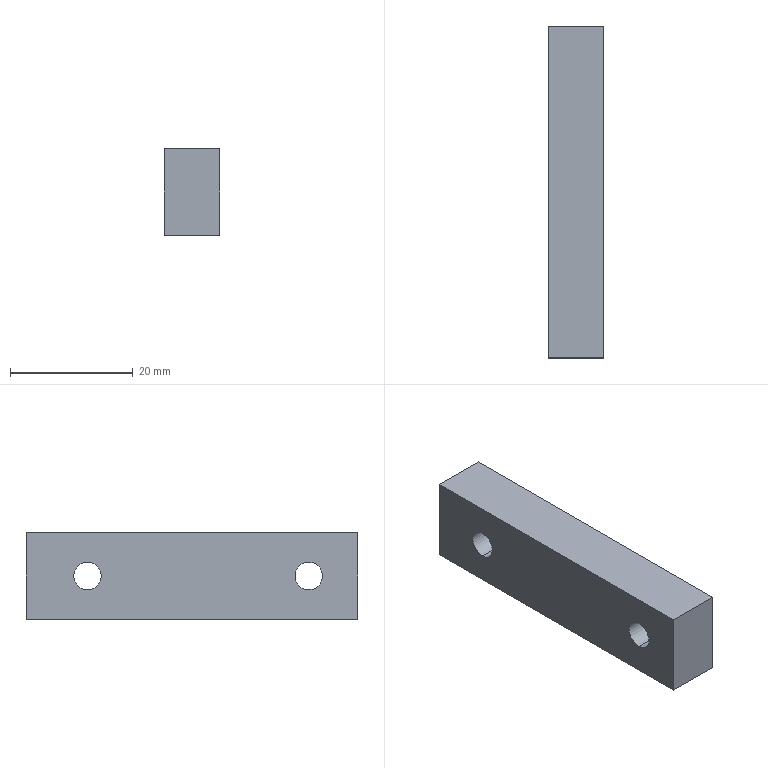Part | STEP file | PN_0004 rubber pad | 1 solid | 16 faces | box 9 x 54 x 14 mm | volume 6202 mm3 | cylinder 8 | plane 8 | commonest cylinder face diameters 4.5 x4 8 x4
STEP:
#1=CARTESIAN_POINT('',(0.,0.,0.));
#2=DIRECTION('',(0.,0.,1.));
#3=DIRECTION('',(1.,0.,0.));
#4=AXIS2_PLACEMENT_3D('',#1,#2,#3);
#5=CARTESIAN_POINT('',(4.4,44.,-4.));
#6=VERTEX_POINT('',#5);
#7=CARTESIAN_POINT('',(9.,44.,-4.));
#8=VERTEX_POINT('',#7);
#9=CARTESIAN_POINT('',(9.,44.,-4.));
#10=DIRECTION('',(1.,0.,0.));
#11=VECTOR('',#10,1.);
#12=LINE('',#9,#11);
#13=CARTESIAN_POINT('',(9.,44.,0.));
#14=DIRECTION('',(1.,0.,0.));
#15=DIRECTION('',(0.,0.,-1.));
#16=AXIS2_PLACEMENT_3D('',#13,#14,#15);
#17=CYLINDRICAL_SURFACE('',#16,4.);
#18=CARTESIAN_POINT('',(6.283,0.));
#19=DIRECTION('',(0.,1.));
#20=VECTOR('',#19,1.);
#21=LINE('',#18,#20);
#22=(GEOMETRIC_REPRESENTATION_CONTEXT(2)PARAMETRIC_REPRESENTATION_CONTEXT()REPRESENTATION_CONTEXT('',''));
#23=DEFINITIONAL_REPRESENTATION('',(#21),#22);
#24=PCURVE('',#17,#23);
#25=CARTESIAN_POINT('',(9.,44.,0.));
#26=DIRECTION('',(1.,0.,0.));
#27=DIRECTION('',(0.,0.,-1.));
#28=AXIS2_PLACEMENT_3D('',#25,#26,#27);
#29=CYLINDRICAL_SURFACE('',#28,4.);
#30=CARTESIAN_POINT('',(0.,0.));
#31=DIRECTION('',(0.,1.));
#32=VECTOR('',#31,1.);
#33=LINE('',#30,#32);
#34=(GEOMETRIC_REPRESENTATION_CONTEXT(2)PARAMETRIC_REPRESENTATION_CONTEXT()REPRESENTATION_CONTEXT('',''));
#35=DEFINITIONAL_REPRESENTATION('',(#33),#34);
#36=PCURVE('',#29,#35);
#37=SURFACE_CURVE('',#12,(#24,#36),.PCURVE_S1.);
#38=EDGE_CURVE('',#6,#8,#37,.T.);
#39=ORIENTED_EDGE('',*,*,#38,.T.);
#40=CARTESIAN_POINT('',(9.,44.,4.));
#41=VERTEX_POINT('',#40);
#42=CARTESIAN_POINT('',(9.,44.,0.));
#43=DIRECTION('',(1.,0.,0.));
#44=DIRECTION('',(0.,0.,-1.));
#45=AXIS2_PLACEMENT_3D('',#42,#43,#44);
#46=CIRCLE('',#45,4.);
#47=CARTESIAN_POINT('',(0.,0.));
#48=DIRECTION('',(1.,0.));
#49=VECTOR('',#48,1.);
#50=LINE('',#47,#49);
#51=(GEOMETRIC_REPRESENTATION_CONTEXT(2)PARAMETRIC_REPRESENTATION_CONTEXT()REPRESENTATION_CONTEXT('',''));
#52=DEFINITIONAL_REPRESENTATION('',(#50),#51);
#53=PCURVE('',#17,#52);
#54=CARTESIAN_POINT('',(9.,0.,0.));
#55=DIRECTION('',(-1.,0.,0.));
#56=DIRECTION('',(0.,0.,1.));
#57=AXIS2_PLACEMENT_3D('',#54,#55,#56);
#58=PLANE('',#57);
#59=CARTESIAN_POINT('',(-4.,44.));
#60=CARTESIAN_POINT('',(-4.,50.928));
#61=CARTESIAN_POINT('',(2.,47.464));
#62=CARTESIAN_POINT('',(8.,44.));
#63=CARTESIAN_POINT('',(2.,40.536));
#64=CARTESIAN_POINT('',(-4.,37.072));
#65=CARTESIAN_POINT('',(-4.,44.));
#66=(BOUNDED_CURVE()B_SPLINE_CURVE(2,(#59,#60,#61,#62,#63,#64,#65),.UNSPECIFIED.,.T.,.F.)B_SPLINE_CURVE_WITH_KNOTS((1,2,2,2,2,1),(-2.094,0.,2.094,4.189,6.283,8.378),.UNSPECIFIED.)CURVE()GEOMETRIC_REPRESENTATION_ITEM()RATIONAL_B_SPLINE_CURVE((1.,0.5,1.,0.5,1.,0.5,1.))REPRESENTATION_ITEM(''));
#67=(GEOMETRIC_REPRESENTATION_CONTEXT(2)PARAMETRIC_REPRESENTATION_CONTEXT()REPRESENTATION_CONTEXT('',''));
#68=DEFINITIONAL_REPRESENTATION('',(#66),#67);
#69=PCURVE('',#58,#68);
#70=SURFACE_CURVE('',#46,(#53,#69),.PCURVE_S1.);
#71=EDGE_CURVE('',#41,#8,#70,.T.);
#72=ORIENTED_EDGE('',*,*,#71,.F.);
#73=CARTESIAN_POINT('',(4.4,44.,4.));
#74=VERTEX_POINT('',#73);
#75=CARTESIAN_POINT('',(9.,44.,4.));
#76=DIRECTION('',(1.,0.,0.));
#77=VECTOR('',#76,1.);
#78=LINE('',#75,#77);
#79=CARTESIAN_POINT('',(3.142,0.));
#80=DIRECTION('',(0.,1.));
#81=VECTOR('',#80,1.);
#82=LINE('',#79,#81);
#83=(GEOMETRIC_REPRESENTATION_CONTEXT(2)PARAMETRIC_REPRESENTATION_CONTEXT()REPRESENTATION_CONTEXT('',''));
#84=DEFINITIONAL_REPRESENTATION('',(#82),#83);
#85=PCURVE('',#17,#84);
#86=CARTESIAN_POINT('',(3.142,0.));
#87=DIRECTION('',(0.,1.));
#88=VECTOR('',#87,1.);
#89=LINE('',#86,#88);
#90=(GEOMETRIC_REPRESENTATION_CONTEXT(2)PARAMETRIC_REPRESENTATION_CONTEXT()REPRESENTATION_CONTEXT('',''));
#91=DEFINITIONAL_REPRESENTATION('',(#89),#90);
#92=PCURVE('',#29,#91);
#93=SURFACE_CURVE('',#78,(#85,#92),.PCURVE_S1.);
#94=EDGE_CURVE('',#74,#41,#93,.T.);
#95=ORIENTED_EDGE('',*,*,#94,.F.);
#96=CARTESIAN_POINT('',(4.4,44.,0.));
#97=DIRECTION('',(1.,0.,0.));
#98=DIRECTION('',(0.,0.,-1.));
#99=AXIS2_PLACEMENT_3D('',#96,#97,#98);
#100=CIRCLE('',#99,4.);
#101=CARTESIAN_POINT('',(0.,-4.6));
#102=DIRECTION('',(1.,0.));
#103=VECTOR('',#102,1.);
#104=LINE('',#101,#103);
#105=(GEOMETRIC_REPRESENTATION_CONTEXT(2)PARAMETRIC_REPRESENTATION_CONTEXT()REPRESENTATION_CONTEXT('',''));
#106=DEFINITIONAL_REPRESENTATION('',(#104),#105);
#107=PCURVE('',#17,#106);
#108=CARTESIAN_POINT('',(4.4,46.25,0.));
#109=DIRECTION('',(-1.,0.,0.));
#110=DIRECTION('',(0.,0.,1.));
#111=AXIS2_PLACEMENT_3D('',#108,#109,#110);
#112=PLANE('',#111);
#113=CARTESIAN_POINT('',(-4.,-2.25));
#114=CARTESIAN_POINT('',(-4.,4.678));
#115=CARTESIAN_POINT('',(2.,1.214));
#116=CARTESIAN_POINT('',(8.,-2.25));
#117=CARTESIAN_POINT('',(2.,-5.714));
#118=CARTESIAN_POINT('',(-4.,-9.178));
#119=CARTESIAN_POINT('',(-4.,-2.25));
#120=(BOUNDED_CURVE()B_SPLINE_CURVE(2,(#113,#114,#115,#116,#117,#118,#119),.UNSPECIFIED.,.T.,.F.)B_SPLINE_CURVE_WITH_KNOTS((1,2,2,2,2,1),(-2.094,0.,2.094,4.189,6.283,8.378),.UNSPECIFIED.)CURVE()GEOMETRIC_REPRESENTATION_ITEM()RATIONAL_B_SPLINE_CURVE((1.,0.5,1.,0.5,1.,0.5,1.))REPRESENTATION_ITEM(''));
#121=(GEOMETRIC_REPRESENTATION_CONTEXT(2)PARAMETRIC_REPRESENTATION_CONTEXT()REPRESENTATION_CONTEXT('',''));
#122=DEFINITIONAL_REPRESENTATION('',(#120),#121);
#123=PCURVE('',#112,#122);
#124=SURFACE_CURVE('',#100,(#107,#123),.PCURVE_S1.);
#125=EDGE_CURVE('',#74,#6,#124,.T.);
#126=ORIENTED_EDGE('',*,*,#125,.T.);
#127=EDGE_LOOP('',(#39,#72,#95,#126));
#128=FACE_BOUND('',#127,.F.);
#129=ADVANCED_FACE('',(#128),#17,.F.);
#130=CARTESIAN_POINT('',(0.,44.,-2.25));
#131=VERTEX_POINT('',#130);
#132=CARTESIAN_POINT('',(4.4,44.,-2.25));
#133=VERTEX_POINT('',#132);
#134=CARTESIAN_POINT('',(9.,44.,-2.25));
#135=DIRECTION('',(1.,0.,0.));
#136=VECTOR('',#135,1.);
#137=LINE('',#134,#136);
#138=CARTESIAN_POINT('',(9.,44.,0.));
#139=DIRECTION('',(1.,0.,0.));
#140=DIRECTION('',(0.,0.,-1.));
#141=AXIS2_PLACEMENT_3D('',#138,#139,#140);
#142=CYLINDRICAL_SURFACE('',#141,2.25);
#143=CARTESIAN_POINT('',(6.283,0.));
#144=DIRECTION('',(0.,1.));
#145=VECTOR('',#144,1.);
#146=LINE('',#143,#145);
#147=(GEOMETRIC_REPRESENTATION_CONTEXT(2)PARAMETRIC_REPRESENTATION_CONTEXT()REPRESENTATION_CONTEXT('',''));
#148=DEFINITIONAL_REPRESENTATION('',(#146),#147);
#149=PCURVE('',#142,#148);
#150=CARTESIAN_POINT('',(9.,44.,0.));
#151=DIRECTION('',(1.,0.,0.));
#152=DIRECTION('',(0.,0.,-1.));
#153=AXIS2_PLACEMENT_3D('',#150,#151,#152);
#154=CYLINDRICAL_SURFACE('',#153,2.25);
#155=CARTESIAN_POINT('',(0.,0.));
#156=DIRECTION('',(0.,1.));
#157=VECTOR('',#156,1.);
#158=LINE('',#155,#157);
#159=(GEOMETRIC_REPRESENTATION_CONTEXT(2)PARAMETRIC_REPRESENTATION_CONTEXT()REPRESENTATION_CONTEXT('',''));
#160=DEFINITIONAL_REPRESENTATION('',(#158),#159);
#161=PCURVE('',#154,#160);
#162=SURFACE_CURVE('',#137,(#149,#161),.PCURVE_S1.);
#163=EDGE_CURVE('',#131,#133,#162,.T.);
#164=ORIENTED_EDGE('',*,*,#163,.T.);
#165=CARTESIAN_POINT('',(4.4,44.,2.25));
#166=VERTEX_POINT('',#165);
#167=CARTESIAN_POINT('',(4.4,44.,0.));
#168=DIRECTION('',(1.,0.,0.));
#169=DIRECTION('',(0.,0.,-1.));
#170=AXIS2_PLACEMENT_3D('',#167,#168,#169);
#171=CIRCLE('',#170,2.25);
#172=CARTESIAN_POINT('',(0.,-4.6));
#173=DIRECTION('',(1.,0.));
#174=VECTOR('',#173,1.);
#175=LINE('',#172,#174);
#176=(GEOMETRIC_REPRESENTATION_CONTEXT(2)PARAMETRIC_REPRESENTATION_CONTEXT()REPRESENTATION_CONTEXT('',''));
#177=DEFINITIONAL_REPRESENTATION('',(#175),#176);
#178=PCURVE('',#142,#177);
#179=CARTESIAN_POINT('',(-2.25,-2.25));
#180=CARTESIAN_POINT('',(-2.25,1.647));
#181=CARTESIAN_POINT('',(1.125,-0.3014));
#182=CARTESIAN_POINT('',(4.5,-2.25));
#183=CARTESIAN_POINT('',(1.125,-4.199));
#184=CARTESIAN_POINT('',(-2.25,-6.147));
#185=CARTESIAN_POINT('',(-2.25,-2.25));
#186=(BOUNDED_CURVE()B_SPLINE_CURVE(2,(#179,#180,#181,#182,#183,#184,#185),.UNSPECIFIED.,.T.,.F.)B_SPLINE_CURVE_WITH_KNOTS((1,2,2,2,2,1),(-2.094,0.,2.094,4.189,6.283,8.378),.UNSPECIFIED.)CURVE()GEOMETRIC_REPRESENTATION_ITEM()RATIONAL_B_SPLINE_CURVE((1.,0.5,1.,0.5,1.,0.5,1.))REPRESENTATION_ITEM(''));
#187=(GEOMETRIC_REPRESENTATION_CONTEXT(2)PARAMETRIC_REPRESENTATION_CONTEXT()REPRESENTATION_CONTEXT('',''));
#188=DEFINITIONAL_REPRESENTATION('',(#186),#187);
#189=PCURVE('',#112,#188);
#190=SURFACE_CURVE('',#171,(#178,#189),.PCURVE_S1.);
#191=EDGE_CURVE('',#166,#133,#190,.T.);
#192=ORIENTED_EDGE('',*,*,#191,.F.);
#193=CARTESIAN_POINT('',(0.,44.,2.25));
#194=VERTEX_POINT('',#193);
#195=CARTESIAN_POINT('',(9.,44.,2.25));
#196=DIRECTION('',(1.,0.,0.));
#197=VECTOR('',#196,1.);
#198=LINE('',#195,#197);
#199=CARTESIAN_POINT('',(3.142,0.));
#200=DIRECTION('',(0.,1.));
#201=VECTOR('',#200,1.);
#202=LINE('',#199,#201);
#203=(GEOMETRIC_REPRESENTATION_CONTEXT(2)PARAMETRIC_REPRESENTATION_CONTEXT()REPRESENTATION_CONTEXT('',''));
#204=DEFINITIONAL_REPRESENTATION('',(#202),#203);
#205=PCURVE('',#142,#204);
#206=CARTESIAN_POINT('',(3.142,0.));
#207=DIRECTION('',(0.,1.));
#208=VECTOR('',#207,1.);
#209=LINE('',#206,#208);
#210=(GEOMETRIC_REPRESENTATION_CONTEXT(2)PARAMETRIC_REPRESENTATION_CONTEXT()REPRESENTATION_CONTEXT('',''));
#211=DEFINITIONAL_REPRESENTATION('',(#209),#210);
#212=PCURVE('',#154,#211);
#213=SURFACE_CURVE('',#198,(#205,#212),.PCURVE_S1.);
#214=EDGE_CURVE('',#194,#166,#213,.T.);
#215=ORIENTED_EDGE('',*,*,#214,.F.);
#216=CARTESIAN_POINT('',(0.,44.,0.));
#217=DIRECTION('',(1.,0.,0.));
#218=DIRECTION('',(0.,0.,-1.));
#219=AXIS2_PLACEMENT_3D('',#216,#217,#218);
#220=CIRCLE('',#219,2.25);
#221=CARTESIAN_POINT('',(0.,-9.));
#222=DIRECTION('',(1.,0.));
#223=VECTOR('',#222,1.);
#224=LINE('',#221,#223);
#225=(GEOMETRIC_REPRESENTATION_CONTEXT(2)PARAMETRIC_REPRESENTATION_CONTEXT()REPRESENTATION_CONTEXT('',''));
#226=DEFINITIONAL_REPRESENTATION('',(#224),#225);
#227=PCURVE('',#142,#226);
#228=CARTESIAN_POINT('',(0.,0.,0.));
#229=DIRECTION('',(-1.,0.,0.));
#230=DIRECTION('',(0.,0.,1.));
#231=AXIS2_PLACEMENT_3D('',#228,#229,#230);
#232=PLANE('',#231);
#233=CARTESIAN_POINT('',(-2.25,44.));
#234=CARTESIAN_POINT('',(-2.25,47.897));
#235=CARTESIAN_POINT('',(1.125,45.949));
#236=CARTESIAN_POINT('',(4.5,44.));
#237=CARTESIAN_POINT('',(1.125,42.051));
#238=CARTESIAN_POINT('',(-2.25,40.103));
#239=CARTESIAN_POINT('',(-2.25,44.));
#240=(BOUNDED_CURVE()B_SPLINE_CURVE(2,(#233,#234,#235,#236,#237,#238,#239),.UNSPECIFIED.,.T.,.F.)B_SPLINE_CURVE_WITH_KNOTS((1,2,2,2,2,1),(-2.094,0.,2.094,4.189,6.283,8.378),.UNSPECIFIED.)CURVE()GEOMETRIC_REPRESENTATION_ITEM()RATIONAL_B_SPLINE_CURVE((1.,0.5,1.,0.5,1.,0.5,1.))REPRESENTATION_ITEM(''));
#241=(GEOMETRIC_REPRESENTATION_CONTEXT(2)PARAMETRIC_REPRESENTATION_CONTEXT()REPRESENTATION_CONTEXT('',''));
#242=DEFINITIONAL_REPRESENTATION('',(#240),#241);
#243=PCURVE('',#232,#242);
#244=SURFACE_CURVE('',#220,(#227,#243),.PCURVE_S1.);
#245=EDGE_CURVE('',#194,#131,#244,.T.);
#246=ORIENTED_EDGE('',*,*,#245,.T.);
#247=EDGE_LOOP('',(#164,#192,#215,#246));
#248=FACE_BOUND('',#247,.F.);
#249=ADVANCED_FACE('',(#248),#142,.F.);
#250=CARTESIAN_POINT('',(4.4,8.,-4.));
#251=VERTEX_POINT('',#250);
#252=CARTESIAN_POINT('',(9.,8.,-4.));
#253=VERTEX_POINT('',#252);
#254=CARTESIAN_POINT('',(9.,8.,-4.));
#255=DIRECTION('',(1.,0.,0.));
#256=VECTOR('',#255,1.);
#257=LINE('',#254,#256);
#258=CARTESIAN_POINT('',(9.,8.,0.));
#259=DIRECTION('',(1.,0.,0.));
#260=DIRECTION('',(0.,0.,-1.));
#261=AXIS2_PLACEMENT_3D('',#258,#259,#260);
#262=CYLINDRICAL_SURFACE('',#261,4.);
#263=CARTESIAN_POINT('',(6.283,0.));
#264=DIRECTION('',(0.,1.));
#265=VECTOR('',#264,1.);
#266=LINE('',#263,#265);
#267=(GEOMETRIC_REPRESENTATION_CONTEXT(2)PARAMETRIC_REPRESENTATION_CONTEXT()REPRESENTATION_CONTEXT('',''));
#268=DEFINITIONAL_REPRESENTATION('',(#266),#267);
#269=PCURVE('',#262,#268);
#270=CARTESIAN_POINT('',(9.,8.,0.));
#271=DIRECTION('',(1.,0.,0.));
#272=DIRECTION('',(0.,0.,-1.));
#273=AXIS2_PLACEMENT_3D('',#270,#271,#272);
#274=CYLINDRICAL_SURFACE('',#273,4.);
#275=CARTESIAN_POINT('',(0.,0.));
#276=DIRECTION('',(0.,1.));
#277=VECTOR('',#276,1.);
#278=LINE('',#275,#277);
#279=(GEOMETRIC_REPRESENTATION_CONTEXT(2)PARAMETRIC_REPRESENTATION_CONTEXT()REPRESENTATION_CONTEXT('',''));
#280=DEFINITIONAL_REPRESENTATION('',(#278),#279);
#281=PCURVE('',#274,#280);
#282=SURFACE_CURVE('',#257,(#269,#281),.PCURVE_S1.);
#283=EDGE_CURVE('',#251,#253,#282,.T.);
#284=ORIENTED_EDGE('',*,*,#283,.T.);
#285=CARTESIAN_POINT('',(9.,8.,4.));
#286=VERTEX_POINT('',#285);
#287=CARTESIAN_POINT('',(9.,8.,0.));
#288=DIRECTION('',(1.,0.,0.));
#289=DIRECTION('',(0.,0.,-1.));
#290=AXIS2_PLACEMENT_3D('',#287,#288,#289);
#291=CIRCLE('',#290,4.);
#292=CARTESIAN_POINT('',(0.,0.));
#293=DIRECTION('',(1.,0.));
#294=VECTOR('',#293,1.);
#295=LINE('',#292,#294);
#296=(GEOMETRIC_REPRESENTATION_CONTEXT(2)PARAMETRIC_REPRESENTATION_CONTEXT()REPRESENTATION_CONTEXT('',''));
#297=DEFINITIONAL_REPRESENTATION('',(#295),#296);
#298=PCURVE('',#262,#297);
#299=CARTESIAN_POINT('',(-4.,8.));
#300=CARTESIAN_POINT('',(-4.,14.928));
#301=CARTESIAN_POINT('',(2.,11.464));
#302=CARTESIAN_POINT('',(8.,8.));
#303=CARTESIAN_POINT('',(2.,4.536));
#304=CARTESIAN_POINT('',(-4.,1.072));
#305=CARTESIAN_POINT('',(-4.,8.));
#306=(BOUNDED_CURVE()B_SPLINE_CURVE(2,(#299,#300,#301,#302,#303,#304,#305),.UNSPECIFIED.,.T.,.F.)B_SPLINE_CURVE_WITH_KNOTS((1,2,2,2,2,1),(-2.094,0.,2.094,4.189,6.283,8.378),.UNSPECIFIED.)CURVE()GEOMETRIC_REPRESENTATION_ITEM()RATIONAL_B_SPLINE_CURVE((1.,0.5,1.,0.5,1.,0.5,1.))REPRESENTATION_ITEM(''));
#307=(GEOMETRIC_REPRESENTATION_CONTEXT(2)PARAMETRIC_REPRESENTATION_CONTEXT()REPRESENTATION_CONTEXT('',''));
#308=DEFINITIONAL_REPRESENTATION('',(#306),#307);
#309=PCURVE('',#58,#308);
#310=SURFACE_CURVE('',#291,(#298,#309),.PCURVE_S1.);
#311=EDGE_CURVE('',#286,#253,#310,.T.);
#312=ORIENTED_EDGE('',*,*,#311,.F.);
#313=CARTESIAN_POINT('',(4.4,8.,4.));
#314=VERTEX_POINT('',#313);
#315=CARTESIAN_POINT('',(9.,8.,4.));
#316=DIRECTION('',(1.,0.,0.));
#317=VECTOR('',#316,1.);
#318=LINE('',#315,#317);
#319=CARTESIAN_POINT('',(3.142,0.));
#320=DIRECTION('',(0.,1.));
#321=VECTOR('',#320,1.);
#322=LINE('',#319,#321);
#323=(GEOMETRIC_REPRESENTATION_CONTEXT(2)PARAMETRIC_REPRESENTATION_CONTEXT()REPRESENTATION_CONTEXT('',''));
#324=DEFINITIONAL_REPRESENTATION('',(#322),#323);
#325=PCURVE('',#262,#324);
#326=CARTESIAN_POINT('',(3.142,0.));
#327=DIRECTION('',(0.,1.));
#328=VECTOR('',#327,1.);
#329=LINE('',#326,#328);
#330=(GEOMETRIC_REPRESENTATION_CONTEXT(2)PARAMETRIC_REPRESENTATION_CONTEXT()REPRESENTATION_CONTEXT('',''));
#331=DEFINITIONAL_REPRESENTATION('',(#329),#330);
#332=PCURVE('',#274,#331);
#333=SURFACE_CURVE('',#318,(#325,#332),.PCURVE_S1.);
#334=EDGE_CURVE('',#314,#286,#333,.T.);
#335=ORIENTED_EDGE('',*,*,#334,.F.);
#336=CARTESIAN_POINT('',(4.4,8.,0.));
#337=DIRECTION('',(1.,0.,0.));
#338=DIRECTION('',(0.,0.,-1.));
#339=AXIS2_PLACEMENT_3D('',#336,#337,#338);
#340=CIRCLE('',#339,4.);
#341=CARTESIAN_POINT('',(0.,-4.6));
#342=DIRECTION('',(1.,0.));
#343=VECTOR('',#342,1.);
#344=LINE('',#341,#343);
#345=(GEOMETRIC_REPRESENTATION_CONTEXT(2)PARAMETRIC_REPRESENTATION_CONTEXT()REPRESENTATION_CONTEXT('',''));
#346=DEFINITIONAL_REPRESENTATION('',(#344),#345);
#347=PCURVE('',#262,#346);
#348=CARTESIAN_POINT('',(4.4,10.25,0.));
#349=DIRECTION('',(-1.,0.,0.));
#350=DIRECTION('',(0.,0.,1.));
#351=AXIS2_PLACEMENT_3D('',#348,#349,#350);
#352=PLANE('',#351);
#353=CARTESIAN_POINT('',(-4.,-2.25));
#354=CARTESIAN_POINT('',(-4.,4.678));
#355=CARTESIAN_POINT('',(2.,1.214));
#356=CARTESIAN_POINT('',(8.,-2.25));
#357=CARTESIAN_POINT('',(2.,-5.714));
#358=CARTESIAN_POINT('',(-4.,-9.178));
#359=CARTESIAN_POINT('',(-4.,-2.25));
#360=(BOUNDED_CURVE()B_SPLINE_CURVE(2,(#353,#354,#355,#356,#357,#358,#359),.UNSPECIFIED.,.T.,.F.)B_SPLINE_CURVE_WITH_KNOTS((1,2,2,2,2,1),(-2.094,0.,2.094,4.189,6.283,8.378),.UNSPECIFIED.)CURVE()GEOMETRIC_REPRESENTATION_ITEM()RATIONAL_B_SPLINE_CURVE((1.,0.5,1.,0.5,1.,0.5,1.))REPRESENTATION_ITEM(''));
#361=(GEOMETRIC_REPRESENTATION_CONTEXT(2)PARAMETRIC_REPRESENTATION_CONTEXT()REPRESENTATION_CONTEXT('',''));
#362=DEFINITIONAL_REPRESENTATION('',(#360),#361);
#363=PCURVE('',#352,#362);
#364=SURFACE_CURVE('',#340,(#347,#363),.PCURVE_S1.);
#365=EDGE_CURVE('',#314,#251,#364,.T.);
#366=ORIENTED_EDGE('',*,*,#365,.T.);
#367=EDGE_LOOP('',(#284,#312,#335,#366));
#368=FACE_BOUND('',#367,.F.);
#369=ADVANCED_FACE('',(#368),#262,.F.);
#370=CARTESIAN_POINT('',(0.,8.,-2.25));
#371=VERTEX_POINT('',#370);
#372=CARTESIAN_POINT('',(4.4,8.,-2.25));
#373=VERTEX_POINT('',#372);
#374=CARTESIAN_POINT('',(9.,8.,-2.25));
#375=DIRECTION('',(1.,0.,0.));
#376=VECTOR('',#375,1.);
#377=LINE('',#374,#376);
#378=CARTESIAN_POINT('',(9.,8.,0.));
#379=DIRECTION('',(1.,0.,0.));
#380=DIRECTION('',(0.,0.,-1.));
#381=AXIS2_PLACEMENT_3D('',#378,#379,#380);
#382=CYLINDRICAL_SURFACE('',#381,2.25);
#383=CARTESIAN_POINT('',(6.283,0.));
#384=DIRECTION('',(0.,1.));
#385=VECTOR('',#384,1.);
#386=LINE('',#383,#385);
#387=(GEOMETRIC_REPRESENTATION_CONTEXT(2)PARAMETRIC_REPRESENTATION_CONTEXT()REPRESENTATION_CONTEXT('',''));
#388=DEFINITIONAL_REPRESENTATION('',(#386),#387);
#389=PCURVE('',#382,#388);
#390=CARTESIAN_POINT('',(9.,8.,0.));
#391=DIRECTION('',(1.,0.,0.));
#392=DIRECTION('',(0.,0.,-1.));
#393=AXIS2_PLACEMENT_3D('',#390,#391,#392);
#394=CYLINDRICAL_SURFACE('',#393,2.25);
#395=CARTESIAN_POINT('',(0.,0.));
#396=DIRECTION('',(0.,1.));
#397=VECTOR('',#396,1.);
#398=LINE('',#395,#397);
#399=(GEOMETRIC_REPRESENTATION_CONTEXT(2)PARAMETRIC_REPRESENTATION_CONTEXT()REPRESENTATION_CONTEXT('',''));
#400=DEFINITIONAL_REPRESENTATION('',(#398),#399);
#401=PCURVE('',#394,#400);
#402=SURFACE_CURVE('',#377,(#389,#401),.PCURVE_S1.);
#403=EDGE_CURVE('',#371,#373,#402,.T.);
#404=ORIENTED_EDGE('',*,*,#403,.T.);
#405=CARTESIAN_POINT('',(4.4,8.,2.25));
#406=VERTEX_POINT('',#405);
#407=CARTESIAN_POINT('',(4.4,8.,0.));
#408=DIRECTION('',(1.,0.,0.));
#409=DIRECTION('',(0.,0.,-1.));
#410=AXIS2_PLACEMENT_3D('',#407,#408,#409);
#411=CIRCLE('',#410,2.25);
#412=CARTESIAN_POINT('',(0.,-4.6));
#413=DIRECTION('',(1.,0.));
#414=VECTOR('',#413,1.);
#415=LINE('',#412,#414);
#416=(GEOMETRIC_REPRESENTATION_CONTEXT(2)PARAMETRIC_REPRESENTATION_CONTEXT()REPRESENTATION_CONTEXT('',''));
#417=DEFINITIONAL_REPRESENTATION('',(#415),#416);
#418=PCURVE('',#382,#417);
#419=CARTESIAN_POINT('',(-2.25,-2.25));
#420=CARTESIAN_POINT('',(-2.25,1.647));
#421=CARTESIAN_POINT('',(1.125,-0.3014));
#422=CARTESIAN_POINT('',(4.5,-2.25));
#423=CARTESIAN_POINT('',(1.125,-4.199));
#424=CARTESIAN_POINT('',(-2.25,-6.147));
#425=CARTESIAN_POINT('',(-2.25,-2.25));
#426=(BOUNDED_CURVE()B_SPLINE_CURVE(2,(#419,#420,#421,#422,#423,#424,#425),.UNSPECIFIED.,.T.,.F.)B_SPLINE_CURVE_WITH_KNOTS((1,2,2,2,2,1),(-2.094,0.,2.094,4.189,6.283,8.378),.UNSPECIFIED.)CURVE()GEOMETRIC_REPRESENTATION_ITEM()RATIONAL_B_SPLINE_CURVE((1.,0.5,1.,0.5,1.,0.5,1.))REPRESENTATION_ITEM(''));
#427=(GEOMETRIC_REPRESENTATION_CONTEXT(2)PARAMETRIC_REPRESENTATION_CONTEXT()REPRESENTATION_CONTEXT('',''));
#428=DEFINITIONAL_REPRESENTATION('',(#426),#427);
#429=PCURVE('',#352,#428);
#430=SURFACE_CURVE('',#411,(#418,#429),.PCURVE_S1.);
#431=EDGE_CURVE('',#406,#373,#430,.T.);
#432=ORIENTED_EDGE('',*,*,#431,.F.);
#433=CARTESIAN_POINT('',(0.,8.,2.25));
#434=VERTEX_POINT('',#433);
#435=CARTESIAN_POINT('',(9.,8.,2.25));
#436=DIRECTION('',(1.,0.,0.));
#437=VECTOR('',#436,1.);
#438=LINE('',#435,#437);
#439=CARTESIAN_POINT('',(3.142,0.));
#440=DIRECTION('',(0.,1.));
#441=VECTOR('',#440,1.);
#442=LINE('',#439,#441);
#443=(GEOMETRIC_REPRESENTATION_CONTEXT(2)PARAMETRIC_REPRESENTATION_CONTEXT()REPRESENTATION_CONTEXT('',''));
#444=DEFINITIONAL_REPRESENTATION('',(#442),#443);
#445=PCURVE('',#382,#444);
#446=CARTESIAN_POINT('',(3.142,0.));
#447=DIRECTION('',(0.,1.));
#448=VECTOR('',#447,1.);
#449=LINE('',#446,#448);
#450=(GEOMETRIC_REPRESENTATION_CONTEXT(2)PARAMETRIC_REPRESENTATION_CONTEXT()REPRESENTATION_CONTEXT('',''));
#451=DEFINITIONAL_REPRESENTATION('',(#449),#450);
#452=PCURVE('',#394,#451);
#453=SURFACE_CURVE('',#438,(#445,#452),.PCURVE_S1.);
#454=EDGE_CURVE('',#434,#406,#453,.T.);
#455=ORIENTED_EDGE('',*,*,#454,.F.);
#456=CARTESIAN_POINT('',(0.,8.,0.));
#457=DIRECTION('',(1.,0.,0.));
#458=DIRECTION('',(0.,0.,-1.));
#459=AXIS2_PLACEMENT_3D('',#456,#457,#458);
#460=CIRCLE('',#459,2.25);
#461=CARTESIAN_POINT('',(0.,-9.));
#462=DIRECTION('',(1.,0.));
#463=VECTOR('',#462,1.);
#464=LINE('',#461,#463);
#465=(GEOMETRIC_REPRESENTATION_CONTEXT(2)PARAMETRIC_REPRESENTATION_CONTEXT()REPRESENTATION_CONTEXT('',''));
#466=DEFINITIONAL_REPRESENTATION('',(#464),#465);
#467=PCURVE('',#382,#466);
#468=CARTESIAN_POINT('',(-2.25,8.));
#469=CARTESIAN_POINT('',(-2.25,11.897));
#470=CARTESIAN_POINT('',(1.125,9.949));
#471=CARTESIAN_POINT('',(4.5,8.));
#472=CARTESIAN_POINT('',(1.125,6.051));
#473=CARTESIAN_POINT('',(-2.25,4.103));
#474=CARTESIAN_POINT('',(-2.25,8.));
#475=(BOUNDED_CURVE()B_SPLINE_CURVE(2,(#468,#469,#470,#471,#472,#473,#474),.UNSPECIFIED.,.T.,.F.)B_SPLINE_CURVE_WITH_KNOTS((1,2,2,2,2,1),(-2.094,0.,2.094,4.189,6.283,8.378),.UNSPECIFIED.)CURVE()GEOMETRIC_REPRESENTATION_ITEM()RATIONAL_B_SPLINE_CURVE((1.,0.5,1.,0.5,1.,0.5,1.))REPRESENTATION_ITEM(''));
#476=(GEOMETRIC_REPRESENTATION_CONTEXT(2)PARAMETRIC_REPRESENTATION_CONTEXT()REPRESENTATION_CONTEXT('',''));
#477=DEFINITIONAL_REPRESENTATION('',(#475),#476);
#478=PCURVE('',#232,#477);
#479=SURFACE_CURVE('',#460,(#467,#478),.PCURVE_S1.);
#480=EDGE_CURVE('',#434,#371,#479,.T.);
#481=ORIENTED_EDGE('',*,*,#480,.T.);
#482=EDGE_LOOP('',(#404,#432,#455,#481));
#483=FACE_BOUND('',#482,.F.);
#484=ADVANCED_FACE('',(#483),#382,.F.);
#485=CARTESIAN_POINT('',(0.,54.,7.));
#486=VERTEX_POINT('',#485);
#487=CARTESIAN_POINT('',(0.,0.,7.));
#488=VERTEX_POINT('',#487);
#489=CARTESIAN_POINT('',(0.,0.,7.));
#490=DIRECTION('',(0.,-1.,0.));
#491=VECTOR('',#490,1.);
#492=LINE('',#489,#491);
#493=CARTESIAN_POINT('',(9.,0.,7.));
#494=DIRECTION('',(0.,0.,-1.));
#495=DIRECTION('',(-1.,0.,0.));
#496=AXIS2_PLACEMENT_3D('',#493,#494,#495);
#497=PLANE('',#496);
#498=CARTESIAN_POINT('',(9.,0.));
#499=DIRECTION('',(0.,-1.));
#500=VECTOR('',#499,1.);
#501=LINE('',#498,#500);
#502=(GEOMETRIC_REPRESENTATION_CONTEXT(2)PARAMETRIC_REPRESENTATION_CONTEXT()REPRESENTATION_CONTEXT('',''));
#503=DEFINITIONAL_REPRESENTATION('',(#501),#502);
#504=PCURVE('',#497,#503);
#505=CARTESIAN_POINT('',(7.,0.));
#506=DIRECTION('',(0.,-1.));
#507=VECTOR('',#506,1.);
#508=LINE('',#505,#507);
#509=(GEOMETRIC_REPRESENTATION_CONTEXT(2)PARAMETRIC_REPRESENTATION_CONTEXT()REPRESENTATION_CONTEXT('',''));
#510=DEFINITIONAL_REPRESENTATION('',(#508),#509);
#511=PCURVE('',#232,#510);
#512=SURFACE_CURVE('',#492,(#504,#511),.PCURVE_S1.);
#513=EDGE_CURVE('',#486,#488,#512,.T.);
#514=ORIENTED_EDGE('',*,*,#513,.T.);
#515=CARTESIAN_POINT('',(9.,0.,7.));
#516=VERTEX_POINT('',#515);
#517=CARTESIAN_POINT('',(9.,0.,7.));
#518=DIRECTION('',(-1.,0.,0.));
#519=VECTOR('',#518,1.);
#520=LINE('',#517,#519);
#521=CARTESIAN_POINT('',(0.,0.));
#522=DIRECTION('',(1.,0.));
#523=VECTOR('',#522,1.);
#524=LINE('',#521,#523);
#525=(GEOMETRIC_REPRESENTATION_CONTEXT(2)PARAMETRIC_REPRESENTATION_CONTEXT()REPRESENTATION_CONTEXT('',''));
#526=DEFINITIONAL_REPRESENTATION('',(#524),#525);
#527=PCURVE('',#497,#526);
#528=CARTESIAN_POINT('',(9.,0.,7.));
#529=DIRECTION('',(0.,1.,0.));
#530=DIRECTION('',(0.,0.,1.));
#531=AXIS2_PLACEMENT_3D('',#528,#529,#530);
#532=PLANE('',#531);
#533=CARTESIAN_POINT('',(0.,0.));
#534=DIRECTION('',(0.,-1.));
#535=VECTOR('',#534,1.);
#536=LINE('',#533,#535);
#537=(GEOMETRIC_REPRESENTATION_CONTEXT(2)PARAMETRIC_REPRESENTATION_CONTEXT()REPRESENTATION_CONTEXT('',''));
#538=DEFINITIONAL_REPRESENTATION('',(#536),#537);
#539=PCURVE('',#532,#538);
#540=SURFACE_CURVE('',#520,(#527,#539),.PCURVE_S1.);
#541=EDGE_CURVE('',#516,#488,#540,.T.);
#542=ORIENTED_EDGE('',*,*,#541,.F.);
#543=CARTESIAN_POINT('',(9.,54.,7.));
#544=VERTEX_POINT('',#543);
#545=CARTESIAN_POINT('',(9.,0.,7.));
#546=DIRECTION('',(0.,-1.,0.));
#547=VECTOR('',#546,1.);
#548=LINE('',#545,#547);
#549=CARTESIAN_POINT('',(0.,0.));
#550=DIRECTION('',(0.,-1.));
#551=VECTOR('',#550,1.);
#552=LINE('',#549,#551);
#553=(GEOMETRIC_REPRESENTATION_CONTEXT(2)PARAMETRIC_REPRESENTATION_CONTEXT()REPRESENTATION_CONTEXT('',''));
#554=DEFINITIONAL_REPRESENTATION('',(#552),#553);
#555=PCURVE('',#497,#554);
#556=CARTESIAN_POINT('',(7.,0.));
#557=DIRECTION('',(0.,-1.));
#558=VECTOR('',#557,1.);
#559=LINE('',#556,#558);
#560=(GEOMETRIC_REPRESENTATION_CONTEXT(2)PARAMETRIC_REPRESENTATION_CONTEXT()REPRESENTATION_CONTEXT('',''));
#561=DEFINITIONAL_REPRESENTATION('',(#559),#560);
#562=PCURVE('',#58,#561);
#563=SURFACE_CURVE('',#548,(#555,#562),.PCURVE_S1.);
#564=EDGE_CURVE('',#544,#516,#563,.T.);
#565=ORIENTED_EDGE('',*,*,#564,.F.);
#566=CARTESIAN_POINT('',(9.,54.,7.));
#567=DIRECTION('',(-1.,0.,0.));
#568=VECTOR('',#567,1.);
#569=LINE('',#566,#568);
#570=CARTESIAN_POINT('',(0.,54.));
#571=DIRECTION('',(1.,0.));
#572=VECTOR('',#571,1.);
#573=LINE('',#570,#572);
#574=(GEOMETRIC_REPRESENTATION_CONTEXT(2)PARAMETRIC_REPRESENTATION_CONTEXT()REPRESENTATION_CONTEXT('',''));
#575=DEFINITIONAL_REPRESENTATION('',(#573),#574);
#576=PCURVE('',#497,#575);
#577=CARTESIAN_POINT('',(9.,54.,7.));
#578=DIRECTION('',(0.,-1.,0.));
#579=DIRECTION('',(0.,0.,-1.));
#580=AXIS2_PLACEMENT_3D('',#577,#578,#579);
#581=PLANE('',#580);
#582=CARTESIAN_POINT('',(0.,0.));
#583=DIRECTION('',(0.,-1.));
#584=VECTOR('',#583,1.);
#585=LINE('',#582,#584);
#586=(GEOMETRIC_REPRESENTATION_CONTEXT(2)PARAMETRIC_REPRESENTATION_CONTEXT()REPRESENTATION_CONTEXT('',''));
#587=DEFINITIONAL_REPRESENTATION('',(#585),#586);
#588=PCURVE('',#581,#587);
#589=SURFACE_CURVE('',#569,(#576,#588),.PCURVE_S1.);
#590=EDGE_CURVE('',#544,#486,#589,.T.);
#591=ORIENTED_EDGE('',*,*,#590,.T.);
#592=EDGE_LOOP('',(#514,#542,#565,#591));
#593=FACE_BOUND('',#592,.T.);
#594=ADVANCED_FACE('',(#593),#497,.F.);
#595=CARTESIAN_POINT('',(0.,0.,-7.));
#596=VERTEX_POINT('',#595);
#597=CARTESIAN_POINT('',(0.,0.,7.));
#598=DIRECTION('',(0.,0.,-1.));
#599=VECTOR('',#598,1.);
#600=LINE('',#597,#599);
#601=CARTESIAN_POINT('',(0.,-9.));
#602=DIRECTION('',(-1.,0.));
#603=VECTOR('',#602,1.);
#604=LINE('',#601,#603);
#605=(GEOMETRIC_REPRESENTATION_CONTEXT(2)PARAMETRIC_REPRESENTATION_CONTEXT()REPRESENTATION_CONTEXT('',''));
#606=DEFINITIONAL_REPRESENTATION('',(#604),#605);
#607=PCURVE('',#532,#606);
#608=CARTESIAN_POINT('',(7.,0.));
#609=DIRECTION('',(-1.,0.));
#610=VECTOR('',#609,1.);
#611=LINE('',#608,#610);
#612=(GEOMETRIC_REPRESENTATION_CONTEXT(2)PARAMETRIC_REPRESENTATION_CONTEXT()REPRESENTATION_CONTEXT('',''));
#613=DEFINITIONAL_REPRESENTATION('',(#611),#612);
#614=PCURVE('',#232,#613);
#615=SURFACE_CURVE('',#600,(#607,#614),.PCURVE_S1.);
#616=EDGE_CURVE('',#488,#596,#615,.T.);
#617=ORIENTED_EDGE('',*,*,#616,.T.);
#618=CARTESIAN_POINT('',(9.,0.,-7.));
#619=VERTEX_POINT('',#618);
#620=CARTESIAN_POINT('',(9.,0.,-7.));
#621=DIRECTION('',(-1.,0.,0.));
#622=VECTOR('',#621,1.);
#623=LINE('',#620,#622);
#624=CARTESIAN_POINT('',(-14.,0.));
#625=DIRECTION('',(0.,-1.));
#626=VECTOR('',#625,1.);
#627=LINE('',#624,#626);
#628=(GEOMETRIC_REPRESENTATION_CONTEXT(2)PARAMETRIC_REPRESENTATION_CONTEXT()REPRESENTATION_CONTEXT('',''));
#629=DEFINITIONAL_REPRESENTATION('',(#627),#628);
#630=PCURVE('',#532,#629);
#631=CARTESIAN_POINT('',(9.,0.,-7.));
#632=DIRECTION('',(0.,0.,1.));
#633=DIRECTION('',(1.,0.,0.));
#634=AXIS2_PLACEMENT_3D('',#631,#632,#633);
#635=PLANE('',#634);
#636=CARTESIAN_POINT('',(0.,0.));
#637=DIRECTION('',(-1.,0.));
#638=VECTOR('',#637,1.);
#639=LINE('',#636,#638);
#640=(GEOMETRIC_REPRESENTATION_CONTEXT(2)PARAMETRIC_REPRESENTATION_CONTEXT()REPRESENTATION_CONTEXT('',''));
#641=DEFINITIONAL_REPRESENTATION('',(#639),#640);
#642=PCURVE('',#635,#641);
#643=SURFACE_CURVE('',#623,(#630,#642),.PCURVE_S1.);
#644=EDGE_CURVE('',#619,#596,#643,.T.);
#645=ORIENTED_EDGE('',*,*,#644,.F.);
#646=CARTESIAN_POINT('',(9.,0.,7.));
#647=DIRECTION('',(0.,0.,-1.));
#648=VECTOR('',#647,1.);
#649=LINE('',#646,#648);
#650=CARTESIAN_POINT('',(0.,0.));
#651=DIRECTION('',(-1.,0.));
#652=VECTOR('',#651,1.);
#653=LINE('',#650,#652);
#654=(GEOMETRIC_REPRESENTATION_CONTEXT(2)PARAMETRIC_REPRESENTATION_CONTEXT()REPRESENTATION_CONTEXT('',''));
#655=DEFINITIONAL_REPRESENTATION('',(#653),#654);
#656=PCURVE('',#532,#655);
#657=CARTESIAN_POINT('',(7.,0.));
#658=DIRECTION('',(-1.,0.));
#659=VECTOR('',#658,1.);
#660=LINE('',#657,#659);
#661=(GEOMETRIC_REPRESENTATION_CONTEXT(2)PARAMETRIC_REPRESENTATION_CONTEXT()REPRESENTATION_CONTEXT('',''));
#662=DEFINITIONAL_REPRESENTATION('',(#660),#661);
#663=PCURVE('',#58,#662);
#664=SURFACE_CURVE('',#649,(#656,#663),.PCURVE_S1.);
#665=EDGE_CURVE('',#516,#619,#664,.T.);
#666=ORIENTED_EDGE('',*,*,#665,.F.);
#667=ORIENTED_EDGE('',*,*,#541,.T.);
#668=EDGE_LOOP('',(#617,#645,#666,#667));
#669=FACE_BOUND('',#668,.T.);
#670=ADVANCED_FACE('',(#669),#532,.F.);
#671=CARTESIAN_POINT('',(0.,54.,-7.));
#672=VERTEX_POINT('',#671);
#673=CARTESIAN_POINT('',(0.,0.,-7.));
#674=DIRECTION('',(0.,1.,0.));
#675=VECTOR('',#674,1.);
#676=LINE('',#673,#675);
#677=CARTESIAN_POINT('',(-9.,0.));
#678=DIRECTION('',(0.,1.));
#679=VECTOR('',#678,1.);
#680=LINE('',#677,#679);
#681=(GEOMETRIC_REPRESENTATION_CONTEXT(2)PARAMETRIC_REPRESENTATION_CONTEXT()REPRESENTATION_CONTEXT('',''));
#682=DEFINITIONAL_REPRESENTATION('',(#680),#681);
#683=PCURVE('',#635,#682);
#684=CARTESIAN_POINT('',(-7.,0.));
#685=DIRECTION('',(0.,1.));
#686=VECTOR('',#685,1.);
#687=LINE('',#684,#686);
#688=(GEOMETRIC_REPRESENTATION_CONTEXT(2)PARAMETRIC_REPRESENTATION_CONTEXT()REPRESENTATION_CONTEXT('',''));
#689=DEFINITIONAL_REPRESENTATION('',(#687),#688);
#690=PCURVE('',#232,#689);
#691=SURFACE_CURVE('',#676,(#683,#690),.PCURVE_S1.);
#692=EDGE_CURVE('',#596,#672,#691,.T.);
#693=ORIENTED_EDGE('',*,*,#692,.T.);
#694=CARTESIAN_POINT('',(9.,54.,-7.));
#695=VERTEX_POINT('',#694);
#696=CARTESIAN_POINT('',(9.,54.,-7.));
#697=DIRECTION('',(-1.,0.,0.));
#698=VECTOR('',#697,1.);
#699=LINE('',#696,#698);
#700=CARTESIAN_POINT('',(0.,54.));
#701=DIRECTION('',(-1.,0.));
#702=VECTOR('',#701,1.);
#703=LINE('',#700,#702);
#704=(GEOMETRIC_REPRESENTATION_CONTEXT(2)PARAMETRIC_REPRESENTATION_CONTEXT()REPRESENTATION_CONTEXT('',''));
#705=DEFINITIONAL_REPRESENTATION('',(#703),#704);
#706=PCURVE('',#635,#705);
#707=CARTESIAN_POINT('',(14.,0.));
#708=DIRECTION('',(0.,-1.));
#709=VECTOR('',#708,1.);
#710=LINE('',#707,#709);
#711=(GEOMETRIC_REPRESENTATION_CONTEXT(2)PARAMETRIC_REPRESENTATION_CONTEXT()REPRESENTATION_CONTEXT('',''));
#712=DEFINITIONAL_REPRESENTATION('',(#710),#711);
#713=PCURVE('',#581,#712);
#714=SURFACE_CURVE('',#699,(#706,#713),.PCURVE_S1.);
#715=EDGE_CURVE('',#695,#672,#714,.T.);
#716=ORIENTED_EDGE('',*,*,#715,.F.);
#717=CARTESIAN_POINT('',(9.,0.,-7.));
#718=DIRECTION('',(0.,1.,0.));
#719=VECTOR('',#718,1.);
#720=LINE('',#717,#719);
#721=CARTESIAN_POINT('',(0.,0.));
#722=DIRECTION('',(0.,1.));
#723=VECTOR('',#722,1.);
#724=LINE('',#721,#723);
#725=(GEOMETRIC_REPRESENTATION_CONTEXT(2)PARAMETRIC_REPRESENTATION_CONTEXT()REPRESENTATION_CONTEXT('',''));
#726=DEFINITIONAL_REPRESENTATION('',(#724),#725);
#727=PCURVE('',#635,#726);
#728=CARTESIAN_POINT('',(-7.,0.));
#729=DIRECTION('',(0.,1.));
#730=VECTOR('',#729,1.);
#731=LINE('',#728,#730);
#732=(GEOMETRIC_REPRESENTATION_CONTEXT(2)PARAMETRIC_REPRESENTATION_CONTEXT()REPRESENTATION_CONTEXT('',''));
#733=DEFINITIONAL_REPRESENTATION('',(#731),#732);
#734=PCURVE('',#58,#733);
#735=SURFACE_CURVE('',#720,(#727,#734),.PCURVE_S1.);
#736=EDGE_CURVE('',#619,#695,#735,.T.);
#737=ORIENTED_EDGE('',*,*,#736,.F.);
#738=ORIENTED_EDGE('',*,*,#644,.T.);
#739=EDGE_LOOP('',(#693,#716,#737,#738));
#740=FACE_BOUND('',#739,.T.);
#741=ADVANCED_FACE('',(#740),#635,.F.);
#742=CARTESIAN_POINT('',(0.,54.,7.));
#743=DIRECTION('',(0.,0.,1.));
#744=VECTOR('',#743,1.);
#745=LINE('',#742,#744);
#746=CARTESIAN_POINT('',(0.,-9.));
#747=DIRECTION('',(-1.,0.));
#748=VECTOR('',#747,1.);
#749=LINE('',#746,#748);
#750=(GEOMETRIC_REPRESENTATION_CONTEXT(2)PARAMETRIC_REPRESENTATION_CONTEXT()REPRESENTATION_CONTEXT('',''));
#751=DEFINITIONAL_REPRESENTATION('',(#749),#750);
#752=PCURVE('',#581,#751);
#753=CARTESIAN_POINT('',(7.,54.));
#754=DIRECTION('',(1.,0.));
#755=VECTOR('',#754,1.);
#756=LINE('',#753,#755);
#757=(GEOMETRIC_REPRESENTATION_CONTEXT(2)PARAMETRIC_REPRESENTATION_CONTEXT()REPRESENTATION_CONTEXT('',''));
#758=DEFINITIONAL_REPRESENTATION('',(#756),#757);
#759=PCURVE('',#232,#758);
#760=SURFACE_CURVE('',#745,(#752,#759),.PCURVE_S1.);
#761=EDGE_CURVE('',#672,#486,#760,.T.);
#762=ORIENTED_EDGE('',*,*,#761,.T.);
#763=ORIENTED_EDGE('',*,*,#590,.F.);
#764=CARTESIAN_POINT('',(9.,54.,7.));
#765=DIRECTION('',(0.,0.,1.));
#766=VECTOR('',#765,1.);
#767=LINE('',#764,#766);
#768=CARTESIAN_POINT('',(0.,0.));
#769=DIRECTION('',(-1.,0.));
#770=VECTOR('',#769,1.);
#771=LINE('',#768,#770);
#772=(GEOMETRIC_REPRESENTATION_CONTEXT(2)PARAMETRIC_REPRESENTATION_CONTEXT()REPRESENTATION_CONTEXT('',''));
#773=DEFINITIONAL_REPRESENTATION('',(#771),#772);
#774=PCURVE('',#581,#773);
#775=CARTESIAN_POINT('',(7.,54.));
#776=DIRECTION('',(1.,0.));
#777=VECTOR('',#776,1.);
#778=LINE('',#775,#777);
#779=(GEOMETRIC_REPRESENTATION_CONTEXT(2)PARAMETRIC_REPRESENTATION_CONTEXT()REPRESENTATION_CONTEXT('',''));
#780=DEFINITIONAL_REPRESENTATION('',(#778),#779);
#781=PCURVE('',#58,#780);
#782=SURFACE_CURVE('',#767,(#774,#781),.PCURVE_S1.);
#783=EDGE_CURVE('',#695,#544,#782,.T.);
#784=ORIENTED_EDGE('',*,*,#783,.F.);
#785=ORIENTED_EDGE('',*,*,#715,.T.);
#786=EDGE_LOOP('',(#762,#763,#784,#785));
#787=FACE_BOUND('',#786,.T.);
#788=ADVANCED_FACE('',(#787),#581,.F.);
#789=CARTESIAN_POINT('',(9.,44.,0.));
#790=DIRECTION('',(1.,0.,0.));
#791=DIRECTION('',(0.,0.,-1.));
#792=AXIS2_PLACEMENT_3D('',#789,#790,#791);
#793=CIRCLE('',#792,4.);
#794=CARTESIAN_POINT('',(-4.,44.));
#795=CARTESIAN_POINT('',(-4.,50.928));
#796=CARTESIAN_POINT('',(2.,47.464));
#797=CARTESIAN_POINT('',(8.,44.));
#798=CARTESIAN_POINT('',(2.,40.536));
#799=CARTESIAN_POINT('',(-4.,37.072));
#800=CARTESIAN_POINT('',(-4.,44.));
#801=(BOUNDED_CURVE()B_SPLINE_CURVE(2,(#794,#795,#796,#797,#798,#799,#800),.UNSPECIFIED.,.T.,.F.)B_SPLINE_CURVE_WITH_KNOTS((1,2,2,2,2,1),(-2.094,0.,2.094,4.189,6.283,8.378),.UNSPECIFIED.)CURVE()GEOMETRIC_REPRESENTATION_ITEM()RATIONAL_B_SPLINE_CURVE((1.,0.5,1.,0.5,1.,0.5,1.))REPRESENTATION_ITEM(''));
#802=(GEOMETRIC_REPRESENTATION_CONTEXT(2)PARAMETRIC_REPRESENTATION_CONTEXT()REPRESENTATION_CONTEXT('',''));
#803=DEFINITIONAL_REPRESENTATION('',(#801),#802);
#804=PCURVE('',#58,#803);
#805=CARTESIAN_POINT('',(0.,0.));
#806=DIRECTION('',(1.,0.));
#807=VECTOR('',#806,1.);
#808=LINE('',#805,#807);
#809=(GEOMETRIC_REPRESENTATION_CONTEXT(2)PARAMETRIC_REPRESENTATION_CONTEXT()REPRESENTATION_CONTEXT('',''));
#810=DEFINITIONAL_REPRESENTATION('',(#808),#809);
#811=PCURVE('',#29,#810);
#812=SURFACE_CURVE('',#793,(#804,#811),.PCURVE_S1.);
#813=EDGE_CURVE('',#8,#41,#812,.T.);
#814=ORIENTED_EDGE('',*,*,#813,.F.);
#815=ORIENTED_EDGE('',*,*,#71,.F.);
#816=EDGE_LOOP('',(#814,#815));
#817=FACE_BOUND('',#816,.T.);
#818=CARTESIAN_POINT('',(9.,8.,0.));
#819=DIRECTION('',(1.,0.,0.));
#820=DIRECTION('',(0.,0.,-1.));
#821=AXIS2_PLACEMENT_3D('',#818,#819,#820);
#822=CIRCLE('',#821,4.);
#823=CARTESIAN_POINT('',(-4.,8.));
#824=CARTESIAN_POINT('',(-4.,14.928));
#825=CARTESIAN_POINT('',(2.,11.464));
#826=CARTESIAN_POINT('',(8.,8.));
#827=CARTESIAN_POINT('',(2.,4.536));
#828=CARTESIAN_POINT('',(-4.,1.072));
#829=CARTESIAN_POINT('',(-4.,8.));
#830=(BOUNDED_CURVE()B_SPLINE_CURVE(2,(#823,#824,#825,#826,#827,#828,#829),.UNSPECIFIED.,.T.,.F.)B_SPLINE_CURVE_WITH_KNOTS((1,2,2,2,2,1),(-2.094,0.,2.094,4.189,6.283,8.378),.UNSPECIFIED.)CURVE()GEOMETRIC_REPRESENTATION_ITEM()RATIONAL_B_SPLINE_CURVE((1.,0.5,1.,0.5,1.,0.5,1.))REPRESENTATION_ITEM(''));
#831=(GEOMETRIC_REPRESENTATION_CONTEXT(2)PARAMETRIC_REPRESENTATION_CONTEXT()REPRESENTATION_CONTEXT('',''));
#832=DEFINITIONAL_REPRESENTATION('',(#830),#831);
#833=PCURVE('',#58,#832);
#834=CARTESIAN_POINT('',(0.,0.));
#835=DIRECTION('',(1.,0.));
#836=VECTOR('',#835,1.);
#837=LINE('',#834,#836);
#838=(GEOMETRIC_REPRESENTATION_CONTEXT(2)PARAMETRIC_REPRESENTATION_CONTEXT()REPRESENTATION_CONTEXT('',''));
#839=DEFINITIONAL_REPRESENTATION('',(#837),#838);
#840=PCURVE('',#274,#839);
#841=SURFACE_CURVE('',#822,(#833,#840),.PCURVE_S1.);
#842=EDGE_CURVE('',#253,#286,#841,.T.);
#843=ORIENTED_EDGE('',*,*,#842,.F.);
#844=ORIENTED_EDGE('',*,*,#311,.F.);
#845=EDGE_LOOP('',(#843,#844));
#846=FACE_BOUND('',#845,.T.);
#847=ORIENTED_EDGE('',*,*,#564,.T.);
#848=ORIENTED_EDGE('',*,*,#665,.T.);
#849=ORIENTED_EDGE('',*,*,#736,.T.);
#850=ORIENTED_EDGE('',*,*,#783,.T.);
#851=EDGE_LOOP('',(#847,#848,#849,#850));
#852=FACE_BOUND('',#851,.T.);
#853=ADVANCED_FACE('',(#817,#846,#852),#58,.F.);
#854=CARTESIAN_POINT('',(0.,44.,0.));
#855=DIRECTION('',(1.,0.,0.));
#856=DIRECTION('',(0.,0.,-1.));
#857=AXIS2_PLACEMENT_3D('',#854,#855,#856);
#858=CIRCLE('',#857,2.25);
#859=CARTESIAN_POINT('',(-2.25,44.));
#860=CARTESIAN_POINT('',(-2.25,47.897));
#861=CARTESIAN_POINT('',(1.125,45.949));
#862=CARTESIAN_POINT('',(4.5,44.));
#863=CARTESIAN_POINT('',(1.125,42.051));
#864=CARTESIAN_POINT('',(-2.25,40.103));
#865=CARTESIAN_POINT('',(-2.25,44.));
#866=(BOUNDED_CURVE()B_SPLINE_CURVE(2,(#859,#860,#861,#862,#863,#864,#865),.UNSPECIFIED.,.T.,.F.)B_SPLINE_CURVE_WITH_KNOTS((1,2,2,2,2,1),(-2.094,0.,2.094,4.189,6.283,8.378),.UNSPECIFIED.)CURVE()GEOMETRIC_REPRESENTATION_ITEM()RATIONAL_B_SPLINE_CURVE((1.,0.5,1.,0.5,1.,0.5,1.))REPRESENTATION_ITEM(''));
#867=(GEOMETRIC_REPRESENTATION_CONTEXT(2)PARAMETRIC_REPRESENTATION_CONTEXT()REPRESENTATION_CONTEXT('',''));
#868=DEFINITIONAL_REPRESENTATION('',(#866),#867);
#869=PCURVE('',#232,#868);
#870=CARTESIAN_POINT('',(0.,-9.));
#871=DIRECTION('',(1.,0.));
#872=VECTOR('',#871,1.);
#873=LINE('',#870,#872);
#874=(GEOMETRIC_REPRESENTATION_CONTEXT(2)PARAMETRIC_REPRESENTATION_CONTEXT()REPRESENTATION_CONTEXT('',''));
#875=DEFINITIONAL_REPRESENTATION('',(#873),#874);
#876=PCURVE('',#154,#875);
#877=SURFACE_CURVE('',#858,(#869,#876),.PCURVE_S1.);
#878=EDGE_CURVE('',#131,#194,#877,.T.);
#879=ORIENTED_EDGE('',*,*,#878,.T.);
#880=ORIENTED_EDGE('',*,*,#245,.T.);
#881=EDGE_LOOP('',(#879,#880));
#882=FACE_BOUND('',#881,.T.);
#883=CARTESIAN_POINT('',(0.,8.,0.));
#884=DIRECTION('',(1.,0.,0.));
#885=DIRECTION('',(0.,0.,-1.));
#886=AXIS2_PLACEMENT_3D('',#883,#884,#885);
#887=CIRCLE('',#886,2.25);
#888=CARTESIAN_POINT('',(-2.25,8.));
#889=CARTESIAN_POINT('',(-2.25,11.897));
#890=CARTESIAN_POINT('',(1.125,9.949));
#891=CARTESIAN_POINT('',(4.5,8.));
#892=CARTESIAN_POINT('',(1.125,6.051));
#893=CARTESIAN_POINT('',(-2.25,4.103));
#894=CARTESIAN_POINT('',(-2.25,8.));
#895=(BOUNDED_CURVE()B_SPLINE_CURVE(2,(#888,#889,#890,#891,#892,#893,#894),.UNSPECIFIED.,.T.,.F.)B_SPLINE_CURVE_WITH_KNOTS((1,2,2,2,2,1),(-2.094,0.,2.094,4.189,6.283,8.378),.UNSPECIFIED.)CURVE()GEOMETRIC_REPRESENTATION_ITEM()RATIONAL_B_SPLINE_CURVE((1.,0.5,1.,0.5,1.,0.5,1.))REPRESENTATION_ITEM(''));
#896=(GEOMETRIC_REPRESENTATION_CONTEXT(2)PARAMETRIC_REPRESENTATION_CONTEXT()REPRESENTATION_CONTEXT('',''));
#897=DEFINITIONAL_REPRESENTATION('',(#895),#896);
#898=PCURVE('',#232,#897);
#899=CARTESIAN_POINT('',(0.,-9.));
#900=DIRECTION('',(1.,0.));
#901=VECTOR('',#900,1.);
#902=LINE('',#899,#901);
#903=(GEOMETRIC_REPRESENTATION_CONTEXT(2)PARAMETRIC_REPRESENTATION_CONTEXT()REPRESENTATION_CONTEXT('',''));
#904=DEFINITIONAL_REPRESENTATION('',(#902),#903);
#905=PCURVE('',#394,#904);
#906=SURFACE_CURVE('',#887,(#898,#905),.PCURVE_S1.);
#907=EDGE_CURVE('',#371,#434,#906,.T.);
#908=ORIENTED_EDGE('',*,*,#907,.T.);
#909=ORIENTED_EDGE('',*,*,#480,.T.);
#910=EDGE_LOOP('',(#908,#909));
#911=FACE_BOUND('',#910,.T.);
#912=ORIENTED_EDGE('',*,*,#513,.F.);
#913=ORIENTED_EDGE('',*,*,#761,.F.);
#914=ORIENTED_EDGE('',*,*,#692,.F.);
#915=ORIENTED_EDGE('',*,*,#616,.F.);
#916=EDGE_LOOP('',(#912,#913,#914,#915));
#917=FACE_BOUND('',#916,.T.);
#918=ADVANCED_FACE('',(#882,#911,#917),#232,.T.);
#919=CARTESIAN_POINT('',(4.4,8.,0.));
#920=DIRECTION('',(1.,0.,0.));
#921=DIRECTION('',(0.,0.,-1.));
#922=AXIS2_PLACEMENT_3D('',#919,#920,#921);
#923=CIRCLE('',#922,2.25);
#924=CARTESIAN_POINT('',(0.,-4.6));
#925=DIRECTION('',(1.,0.));
#926=VECTOR('',#925,1.);
#927=LINE('',#924,#926);
#928=(GEOMETRIC_REPRESENTATION_CONTEXT(2)PARAMETRIC_REPRESENTATION_CONTEXT()REPRESENTATION_CONTEXT('',''));
#929=DEFINITIONAL_REPRESENTATION('',(#927),#928);
#930=PCURVE('',#394,#929);
#931=CARTESIAN_POINT('',(-2.25,-2.25));
#932=CARTESIAN_POINT('',(-2.25,1.647));
#933=CARTESIAN_POINT('',(1.125,-0.3014));
#934=CARTESIAN_POINT('',(4.5,-2.25));
#935=CARTESIAN_POINT('',(1.125,-4.199));
#936=CARTESIAN_POINT('',(-2.25,-6.147));
#937=CARTESIAN_POINT('',(-2.25,-2.25));
#938=(BOUNDED_CURVE()B_SPLINE_CURVE(2,(#931,#932,#933,#934,#935,#936,#937),.UNSPECIFIED.,.T.,.F.)B_SPLINE_CURVE_WITH_KNOTS((1,2,2,2,2,1),(-2.094,0.,2.094,4.189,6.283,8.378),.UNSPECIFIED.)CURVE()GEOMETRIC_REPRESENTATION_ITEM()RATIONAL_B_SPLINE_CURVE((1.,0.5,1.,0.5,1.,0.5,1.))REPRESENTATION_ITEM(''));
#939=(GEOMETRIC_REPRESENTATION_CONTEXT(2)PARAMETRIC_REPRESENTATION_CONTEXT()REPRESENTATION_CONTEXT('',''));
#940=DEFINITIONAL_REPRESENTATION('',(#938),#939);
#941=PCURVE('',#352,#940);
#942=SURFACE_CURVE('',#923,(#930,#941),.PCURVE_S1.);
#943=EDGE_CURVE('',#373,#406,#942,.T.);
#944=ORIENTED_EDGE('',*,*,#943,.F.);
#945=ORIENTED_EDGE('',*,*,#403,.F.);
#946=ORIENTED_EDGE('',*,*,#907,.T.);
#947=ORIENTED_EDGE('',*,*,#454,.T.);
#948=EDGE_LOOP('',(#944,#945,#946,#947));
#949=FACE_BOUND('',#948,.F.);
#950=ADVANCED_FACE('',(#949),#394,.F.);
#951=ORIENTED_EDGE('',*,*,#943,.F.);
#952=ORIENTED_EDGE('',*,*,#431,.F.);
#953=EDGE_LOOP('',(#951,#952));
#954=FACE_BOUND('',#953,.T.);
#955=CARTESIAN_POINT('',(4.4,8.,0.));
#956=DIRECTION('',(1.,0.,0.));
#957=DIRECTION('',(0.,0.,-1.));
#958=AXIS2_PLACEMENT_3D('',#955,#956,#957);
#959=CIRCLE('',#958,4.);
#960=CARTESIAN_POINT('',(-4.,-2.25));
#961=CARTESIAN_POINT('',(-4.,4.678));
#962=CARTESIAN_POINT('',(2.,1.214));
#963=CARTESIAN_POINT('',(8.,-2.25));
#964=CARTESIAN_POINT('',(2.,-5.714));
#965=CARTESIAN_POINT('',(-4.,-9.178));
#966=CARTESIAN_POINT('',(-4.,-2.25));
#967=(BOUNDED_CURVE()B_SPLINE_CURVE(2,(#960,#961,#962,#963,#964,#965,#966),.UNSPECIFIED.,.T.,.F.)B_SPLINE_CURVE_WITH_KNOTS((1,2,2,2,2,1),(-2.094,0.,2.094,4.189,6.283,8.378),.UNSPECIFIED.)CURVE()GEOMETRIC_REPRESENTATION_ITEM()RATIONAL_B_SPLINE_CURVE((1.,0.5,1.,0.5,1.,0.5,1.))REPRESENTATION_ITEM(''));
#968=(GEOMETRIC_REPRESENTATION_CONTEXT(2)PARAMETRIC_REPRESENTATION_CONTEXT()REPRESENTATION_CONTEXT('',''));
#969=DEFINITIONAL_REPRESENTATION('',(#967),#968);
#970=PCURVE('',#352,#969);
#971=CARTESIAN_POINT('',(0.,-4.6));
#972=DIRECTION('',(1.,0.));
#973=VECTOR('',#972,1.);
#974=LINE('',#971,#973);
#975=(GEOMETRIC_REPRESENTATION_CONTEXT(2)PARAMETRIC_REPRESENTATION_CONTEXT()REPRESENTATION_CONTEXT('',''));
#976=DEFINITIONAL_REPRESENTATION('',(#974),#975);
#977=PCURVE('',#274,#976);
#978=SURFACE_CURVE('',#959,(#970,#977),.PCURVE_S1.);
#979=EDGE_CURVE('',#251,#314,#978,.T.);
#980=ORIENTED_EDGE('',*,*,#979,.T.);
#981=ORIENTED_EDGE('',*,*,#365,.T.);
#982=EDGE_LOOP('',(#980,#981));
#983=FACE_BOUND('',#982,.T.);
#984=ADVANCED_FACE('',(#954,#983),#352,.F.);
#985=ORIENTED_EDGE('',*,*,#842,.F.);
#986=ORIENTED_EDGE('',*,*,#283,.F.);
#987=ORIENTED_EDGE('',*,*,#979,.T.);
#988=ORIENTED_EDGE('',*,*,#334,.T.);
#989=EDGE_LOOP('',(#985,#986,#987,#988));
#990=FACE_BOUND('',#989,.F.);
#991=ADVANCED_FACE('',(#990),#274,.F.);
#992=CARTESIAN_POINT('',(4.4,44.,0.));
#993=DIRECTION('',(1.,0.,0.));
#994=DIRECTION('',(0.,0.,-1.));
#995=AXIS2_PLACEMENT_3D('',#992,#993,#994);
#996=CIRCLE('',#995,2.25);
#997=CARTESIAN_POINT('',(0.,-4.6));
#998=DIRECTION('',(1.,0.));
#999=VECTOR('',#998,1.);
#1000=LINE('',#997,#999);
#1001=(GEOMETRIC_REPRESENTATION_CONTEXT(2)PARAMETRIC_REPRESENTATION_CONTEXT()REPRESENTATION_CONTEXT('',''));
#1002=DEFINITIONAL_REPRESENTATION('',(#1000),#1001);
#1003=PCURVE('',#154,#1002);
#1004=CARTESIAN_POINT('',(-2.25,-2.25));
#1005=CARTESIAN_POINT('',(-2.25,1.647));
#1006=CARTESIAN_POINT('',(1.125,-0.3014));
#1007=CARTESIAN_POINT('',(4.5,-2.25));
#1008=CARTESIAN_POINT('',(1.125,-4.199));
#1009=CARTESIAN_POINT('',(-2.25,-6.147));
#1010=CARTESIAN_POINT('',(-2.25,-2.25));
#1011=(BOUNDED_CURVE()B_SPLINE_CURVE(2,(#1004,#1005,#1006,#1007,#1008,#1009,#1010),.UNSPECIFIED.,.T.,.F.)B_SPLINE_CURVE_WITH_KNOTS((1,2,2,2,2,1),(-2.094,0.,2.094,4.189,6.283,8.378),.UNSPECIFIED.)CURVE()GEOMETRIC_REPRESENTATION_ITEM()RATIONAL_B_SPLINE_CURVE((1.,0.5,1.,0.5,1.,0.5,1.))REPRESENTATION_ITEM(''));
#1012=(GEOMETRIC_REPRESENTATION_CONTEXT(2)PARAMETRIC_REPRESENTATION_CONTEXT()REPRESENTATION_CONTEXT('',''));
#1013=DEFINITIONAL_REPRESENTATION('',(#1011),#1012);
#1014=PCURVE('',#112,#1013);
#1015=SURFACE_CURVE('',#996,(#1003,#1014),.PCURVE_S1.);
#1016=EDGE_CURVE('',#133,#166,#1015,.T.);
#1017=ORIENTED_EDGE('',*,*,#1016,.F.);
#1018=ORIENTED_EDGE('',*,*,#163,.F.);
#1019=ORIENTED_EDGE('',*,*,#878,.T.);
#1020=ORIENTED_EDGE('',*,*,#214,.T.);
#1021=EDGE_LOOP('',(#1017,#1018,#1019,#1020));
#1022=FACE_BOUND('',#1021,.F.);
#1023=ADVANCED_FACE('',(#1022),#154,.F.);
#1024=ORIENTED_EDGE('',*,*,#1016,.F.);
#1025=ORIENTED_EDGE('',*,*,#191,.F.);
#1026=EDGE_LOOP('',(#1024,#1025));
#1027=FACE_BOUND('',#1026,.T.);
#1028=CARTESIAN_POINT('',(4.4,44.,0.));
#1029=DIRECTION('',(1.,0.,0.));
#1030=DIRECTION('',(0.,0.,-1.));
#1031=AXIS2_PLACEMENT_3D('',#1028,#1029,#1030);
#1032=CIRCLE('',#1031,4.);
#1033=CARTESIAN_POINT('',(-4.,-2.25));
#1034=CARTESIAN_POINT('',(-4.,4.678));
#1035=CARTESIAN_POINT('',(2.,1.214));
#1036=CARTESIAN_POINT('',(8.,-2.25));
#1037=CARTESIAN_POINT('',(2.,-5.714));
#1038=CARTESIAN_POINT('',(-4.,-9.178));
#1039=CARTESIAN_POINT('',(-4.,-2.25));
#1040=(BOUNDED_CURVE()B_SPLINE_CURVE(2,(#1033,#1034,#1035,#1036,#1037,#1038,#1039),.UNSPECIFIED.,.T.,.F.)B_SPLINE_CURVE_WITH_KNOTS((1,2,2,2,2,1),(-2.094,0.,2.094,4.189,6.283,8.378),.UNSPECIFIED.)CURVE()GEOMETRIC_REPRESENTATION_ITEM()RATIONAL_B_SPLINE_CURVE((1.,0.5,1.,0.5,1.,0.5,1.))REPRESENTATION_ITEM(''));
#1041=(GEOMETRIC_REPRESENTATION_CONTEXT(2)PARAMETRIC_REPRESENTATION_CONTEXT()REPRESENTATION_CONTEXT('',''));
#1042=DEFINITIONAL_REPRESENTATION('',(#1040),#1041);
#1043=PCURVE('',#112,#1042);
#1044=CARTESIAN_POINT('',(0.,-4.6));
#1045=DIRECTION('',(1.,0.));
#1046=VECTOR('',#1045,1.);
#1047=LINE('',#1044,#1046);
#1048=(GEOMETRIC_REPRESENTATION_CONTEXT(2)PARAMETRIC_REPRESENTATION_CONTEXT()REPRESENTATION_CONTEXT('',''));
#1049=DEFINITIONAL_REPRESENTATION('',(#1047),#1048);
#1050=PCURVE('',#29,#1049);
#1051=SURFACE_CURVE('',#1032,(#1043,#1050),.PCURVE_S1.);
#1052=EDGE_CURVE('',#6,#74,#1051,.T.);
#1053=ORIENTED_EDGE('',*,*,#1052,.T.);
#1054=ORIENTED_EDGE('',*,*,#125,.T.);
#1055=EDGE_LOOP('',(#1053,#1054));
#1056=FACE_BOUND('',#1055,.T.);
#1057=ADVANCED_FACE('',(#1027,#1056),#112,.F.);
#1058=ORIENTED_EDGE('',*,*,#813,.F.);
#1059=ORIENTED_EDGE('',*,*,#38,.F.);
#1060=ORIENTED_EDGE('',*,*,#1052,.T.);
#1061=ORIENTED_EDGE('',*,*,#94,.T.);
#1062=EDGE_LOOP('',(#1058,#1059,#1060,#1061));
#1063=FACE_BOUND('',#1062,.F.);
#1064=ADVANCED_FACE('',(#1063),#29,.F.);
#1065=CLOSED_SHELL('',(#129,#249,#369,#484,#594,#670,#741,#788,#853,#918,#950,#984,#991,#1023,#1057,#1064));
#1066=MANIFOLD_SOLID_BREP('',#1065);
#1067=(LENGTH_UNIT()NAMED_UNIT(*)SI_UNIT(.MILLI.,.METRE.));
#1068=UNCERTAINTY_MEASURE_WITH_UNIT(LENGTH_MEASURE(0.0000001),#1067,'','');
#1069=(NAMED_UNIT(*)PLANE_ANGLE_UNIT()SI_UNIT($,.RADIAN.));
#1070=(NAMED_UNIT(*)SI_UNIT($,.STERADIAN.)SOLID_ANGLE_UNIT());
#1071=(GEOMETRIC_REPRESENTATION_CONTEXT(3)GLOBAL_UNCERTAINTY_ASSIGNED_CONTEXT((#1068))GLOBAL_UNIT_ASSIGNED_CONTEXT((#1067,#1069,#1070))REPRESENTATION_CONTEXT('',''));
#1072=ADVANCED_BREP_SHAPE_REPRESENTATION('',(#4,#1066),#1071);